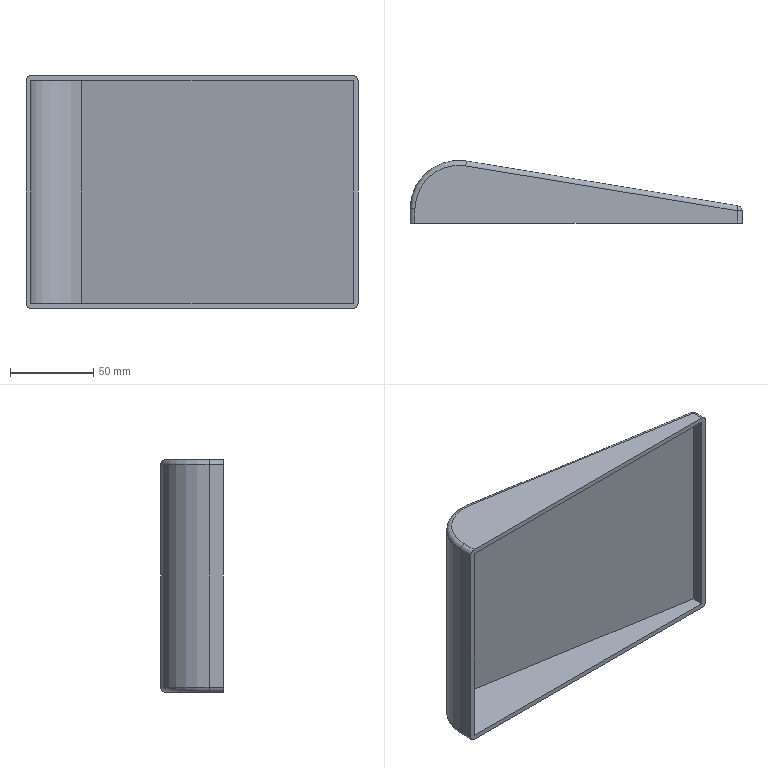Part | SolidWorks | features BaseBody 1 | 1 solid | 24 faces | box 200 x 37.759 x 140 mm | volume 122488 mm3 | plane 11 | cylinder 9 | torus 2 | sphere 2 | commonest cylinder face diameters 6 x7 52.553 x1 58.553 x1
STEP:
#1=CARTESIAN_POINT('',(200.,0.,137.));
#2=VERTEX_POINT('',#1);
#3=CARTESIAN_POINT('',(200.,0.,3.));
#4=VERTEX_POINT('',#3);
#5=CARTESIAN_POINT('',(200.,0.,140.));
#6=DIRECTION('',(0.,0.,-1.));
#7=VECTOR('',#6,1000.);
#8=LINE('',#5,#7);
#9=EDGE_CURVE('',#2,#4,#8,.T.);
#10=ORIENTED_EDGE('',*,*,#9,.F.);
#11=CARTESIAN_POINT('',(197.,0.,140.));
#12=VERTEX_POINT('',#11);
#13=CARTESIAN_POINT('',(197.,0.,137.));
#14=DIRECTION('',(0.,-1.,0.));
#15=DIRECTION('',(-1.,0.,0.));
#16=AXIS2_PLACEMENT_3D('',#13,#14,#15);
#17=CIRCLE('',#16,3.);
#18=EDGE_CURVE('',#2,#12,#17,.T.);
#19=ORIENTED_EDGE('',*,*,#18,.T.);
#20=CARTESIAN_POINT('',(3.,0.,140.));
#21=VERTEX_POINT('',#20);
#22=CARTESIAN_POINT('',(200.,0.,140.));
#23=DIRECTION('',(1.,0.,0.));
#24=VECTOR('',#23,1000.);
#25=LINE('',#22,#24);
#26=EDGE_CURVE('',#21,#12,#25,.T.);
#27=ORIENTED_EDGE('',*,*,#26,.F.);
#28=CARTESIAN_POINT('',(0.,0.,137.));
#29=VERTEX_POINT('',#28);
#30=CARTESIAN_POINT('',(3.,0.,137.));
#31=DIRECTION('',(0.,-1.,0.));
#32=DIRECTION('',(-1.,0.,0.));
#33=AXIS2_PLACEMENT_3D('',#30,#31,#32);
#34=CIRCLE('',#33,3.);
#35=EDGE_CURVE('',#21,#29,#34,.T.);
#36=ORIENTED_EDGE('',*,*,#35,.T.);
#37=CARTESIAN_POINT('',(0.,0.,3.));
#38=VERTEX_POINT('',#37);
#39=CARTESIAN_POINT('',(0.,0.,140.));
#40=DIRECTION('',(0.,0.,-1.));
#41=VECTOR('',#40,1000.);
#42=LINE('',#39,#41);
#43=EDGE_CURVE('',#29,#38,#42,.T.);
#44=ORIENTED_EDGE('',*,*,#43,.T.);
#45=CARTESIAN_POINT('',(3.,0.,0.));
#46=VERTEX_POINT('',#45);
#47=CARTESIAN_POINT('',(3.,0.,3.));
#48=DIRECTION('',(0.,-1.,0.));
#49=DIRECTION('',(-1.,0.,0.));
#50=AXIS2_PLACEMENT_3D('',#47,#48,#49);
#51=CIRCLE('',#50,3.);
#52=EDGE_CURVE('',#38,#46,#51,.T.);
#53=ORIENTED_EDGE('',*,*,#52,.T.);
#54=CARTESIAN_POINT('',(197.,0.,0.));
#55=VERTEX_POINT('',#54);
#56=CARTESIAN_POINT('',(200.,0.,0.));
#57=DIRECTION('',(1.,0.,0.));
#58=VECTOR('',#57,1000.);
#59=LINE('',#56,#58);
#60=EDGE_CURVE('',#46,#55,#59,.T.);
#61=ORIENTED_EDGE('',*,*,#60,.T.);
#62=CARTESIAN_POINT('',(197.,0.,3.));
#63=DIRECTION('',(0.,-1.,0.));
#64=DIRECTION('',(-1.,0.,0.));
#65=AXIS2_PLACEMENT_3D('',#62,#63,#64);
#66=CIRCLE('',#65,3.);
#67=EDGE_CURVE('',#55,#4,#66,.T.);
#68=ORIENTED_EDGE('',*,*,#67,.T.);
#69=EDGE_LOOP('',(#10,#19,#27,#36,#44,#53,#61,#68));
#70=FACE_OUTER_BOUND('',#69,.T.);
#71=CARTESIAN_POINT('',(3.,0.,3.));
#72=VERTEX_POINT('',#71);
#73=CARTESIAN_POINT('',(197.,0.,3.));
#74=VERTEX_POINT('',#73);
#75=CARTESIAN_POINT('',(29.276,0.,3.));
#76=DIRECTION('',(1.,0.,0.));
#77=VECTOR('',#76,1000.);
#78=LINE('',#75,#77);
#79=EDGE_CURVE('',#72,#74,#78,.T.);
#80=ORIENTED_EDGE('',*,*,#79,.F.);
#81=CARTESIAN_POINT('',(3.,0.,137.));
#82=VERTEX_POINT('',#81);
#83=CARTESIAN_POINT('',(3.,0.,140.));
#84=DIRECTION('',(0.,0.,-1.));
#85=VECTOR('',#84,1000.);
#86=LINE('',#83,#85);
#87=EDGE_CURVE('',#82,#72,#86,.T.);
#88=ORIENTED_EDGE('',*,*,#87,.F.);
#89=CARTESIAN_POINT('',(197.,0.,137.));
#90=VERTEX_POINT('',#89);
#91=CARTESIAN_POINT('',(29.276,0.,137.));
#92=DIRECTION('',(1.,0.,0.));
#93=VECTOR('',#92,1000.);
#94=LINE('',#91,#93);
#95=EDGE_CURVE('',#82,#90,#94,.T.);
#96=ORIENTED_EDGE('',*,*,#95,.T.);
#97=CARTESIAN_POINT('',(197.,0.,140.));
#98=DIRECTION('',(0.,0.,-1.));
#99=VECTOR('',#98,1000.);
#100=LINE('',#97,#99);
#101=EDGE_CURVE('',#90,#74,#100,.T.);
#102=ORIENTED_EDGE('',*,*,#101,.T.);
#103=EDGE_LOOP('',(#80,#88,#96,#102));
#104=FACE_BOUND('',#103,.T.);
#105=CARTESIAN_POINT('',(200.,0.,140.));
#106=DIRECTION('',(0.,1.,0.));
#107=DIRECTION('',(-1.,0.,0.));
#108=AXIS2_PLACEMENT_3D('',#105,#106,#107);
#109=PLANE('',#108);
#110=ADVANCED_FACE('',(#70,#104),#109,.F.);
#111=CARTESIAN_POINT('',(200.,7.454,3.));
#112=VERTEX_POINT('',#111);
#113=CARTESIAN_POINT('',(200.,7.454,137.));
#114=VERTEX_POINT('',#113);
#115=CARTESIAN_POINT('',(200.,7.454,140.));
#116=DIRECTION('',(0.,0.,1.));
#117=VECTOR('',#116,1000.);
#118=LINE('',#115,#117);
#119=EDGE_CURVE('',#112,#114,#118,.T.);
#120=ORIENTED_EDGE('',*,*,#119,.T.);
#121=CARTESIAN_POINT('',(200.,10.,137.));
#122=DIRECTION('',(0.,-1.,0.));
#123=VECTOR('',#122,1000.);
#124=LINE('',#121,#123);
#125=EDGE_CURVE('',#114,#2,#124,.T.);
#126=ORIENTED_EDGE('',*,*,#125,.T.);
#127=ORIENTED_EDGE('',*,*,#9,.T.);
#128=CARTESIAN_POINT('',(200.,7.454,3.));
#129=DIRECTION('',(0.,1.,0.));
#130=VECTOR('',#129,1000.);
#131=LINE('',#128,#130);
#132=EDGE_CURVE('',#4,#112,#131,.T.);
#133=ORIENTED_EDGE('',*,*,#132,.T.);
#134=EDGE_LOOP('',(#120,#126,#127,#133));
#135=FACE_OUTER_BOUND('',#134,.T.);
#136=CARTESIAN_POINT('',(200.,10.,140.));
#137=DIRECTION('',(-1.,0.,0.));
#138=DIRECTION('',(0.,0.,1.));
#139=AXIS2_PLACEMENT_3D('',#136,#137,#138);
#140=PLANE('',#139);
#141=ADVANCED_FACE('',(#135),#140,.F.);
#142=CARTESIAN_POINT('',(34.04,37.369,137.));
#143=VERTEX_POINT('',#142);
#144=CARTESIAN_POINT('',(34.04,37.369,3.));
#145=VERTEX_POINT('',#144);
#146=CARTESIAN_POINT('',(34.04,37.369,140.));
#147=DIRECTION('',(0.,0.,-1.));
#148=VECTOR('',#147,1000.);
#149=LINE('',#146,#148);
#150=EDGE_CURVE('',#143,#145,#149,.T.);
#151=ORIENTED_EDGE('',*,*,#150,.F.);
#152=CARTESIAN_POINT('',(197.488,10.414,137.));
#153=VERTEX_POINT('',#152);
#154=CARTESIAN_POINT('',(34.04,37.369,137.));
#155=DIRECTION('',(0.9867,-0.1627,0.));
#156=VECTOR('',#155,1000.);
#157=LINE('',#154,#156);
#158=EDGE_CURVE('',#143,#153,#157,.T.);
#159=ORIENTED_EDGE('',*,*,#158,.T.);
#160=CARTESIAN_POINT('',(197.488,10.414,3.));
#161=VERTEX_POINT('',#160);
#162=CARTESIAN_POINT('',(197.488,10.414,140.));
#163=DIRECTION('',(0.,0.,-1.));
#164=VECTOR('',#163,1000.);
#165=LINE('',#162,#164);
#166=EDGE_CURVE('',#153,#161,#165,.T.);
#167=ORIENTED_EDGE('',*,*,#166,.T.);
#168=CARTESIAN_POINT('',(34.04,37.369,3.));
#169=DIRECTION('',(-0.9867,0.1627,0.));
#170=VECTOR('',#169,1000.);
#171=LINE('',#168,#170);
#172=EDGE_CURVE('',#161,#145,#171,.T.);
#173=ORIENTED_EDGE('',*,*,#172,.T.);
#174=EDGE_LOOP('',(#151,#159,#167,#173));
#175=FACE_OUTER_BOUND('',#174,.T.);
#176=CARTESIAN_POINT('',(34.04,37.369,140.));
#177=DIRECTION('',(-0.1627,-0.9867,0.));
#178=DIRECTION('',(0.9867,-0.1627,0.));
#179=AXIS2_PLACEMENT_3D('',#176,#177,#178);
#180=PLANE('',#179);
#181=ADVANCED_FACE('',(#175),#180,.F.);
#182=CARTESIAN_POINT('',(0.,8.482,137.));
#183=VERTEX_POINT('',#182);
#184=CARTESIAN_POINT('',(0.,8.482,3.));
#185=VERTEX_POINT('',#184);
#186=CARTESIAN_POINT('',(0.,8.482,140.));
#187=DIRECTION('',(0.,0.,-1.));
#188=VECTOR('',#187,1000.);
#189=LINE('',#186,#188);
#190=EDGE_CURVE('',#183,#185,#189,.T.);
#191=ORIENTED_EDGE('',*,*,#190,.F.);
#192=CARTESIAN_POINT('',(29.276,8.482,137.));
#193=DIRECTION('',(0.,0.,-1.));
#194=DIRECTION('',(-1.,0.,0.));
#195=AXIS2_PLACEMENT_3D('',#192,#193,#194);
#196=CIRCLE('',#195,29.276);
#197=EDGE_CURVE('',#183,#143,#196,.T.);
#198=ORIENTED_EDGE('',*,*,#197,.T.);
#199=ORIENTED_EDGE('',*,*,#150,.T.);
#200=CARTESIAN_POINT('',(29.276,8.482,3.));
#201=DIRECTION('',(0.,0.,1.));
#202=DIRECTION('',(-1.,0.,0.));
#203=AXIS2_PLACEMENT_3D('',#200,#201,#202);
#204=CIRCLE('',#203,29.276);
#205=EDGE_CURVE('',#145,#185,#204,.T.);
#206=ORIENTED_EDGE('',*,*,#205,.T.);
#207=EDGE_LOOP('',(#191,#198,#199,#206));
#208=FACE_OUTER_BOUND('',#207,.T.);
#209=CARTESIAN_POINT('',(29.276,8.482,140.));
#210=DIRECTION('',(0.,0.,-1.));
#211=DIRECTION('',(-1.,0.,0.));
#212=AXIS2_PLACEMENT_3D('',#209,#210,#211);
#213=CYLINDRICAL_SURFACE('',#212,29.276);
#214=ADVANCED_FACE('',(#208),#213,.T.);
#215=ORIENTED_EDGE('',*,*,#43,.F.);
#216=CARTESIAN_POINT('',(0.,0.,137.));
#217=DIRECTION('',(0.,1.,0.));
#218=VECTOR('',#217,1000.);
#219=LINE('',#216,#218);
#220=EDGE_CURVE('',#29,#183,#219,.T.);
#221=ORIENTED_EDGE('',*,*,#220,.T.);
#222=ORIENTED_EDGE('',*,*,#190,.T.);
#223=CARTESIAN_POINT('',(0.,0.,3.));
#224=DIRECTION('',(0.,-1.,0.));
#225=VECTOR('',#224,1000.);
#226=LINE('',#223,#225);
#227=EDGE_CURVE('',#185,#38,#226,.T.);
#228=ORIENTED_EDGE('',*,*,#227,.T.);
#229=EDGE_LOOP('',(#215,#221,#222,#228));
#230=FACE_OUTER_BOUND('',#229,.T.);
#231=CARTESIAN_POINT('',(0.,0.,140.));
#232=DIRECTION('',(1.,0.,0.));
#233=DIRECTION('',(0.,0.,-1.));
#234=AXIS2_PLACEMENT_3D('',#231,#232,#233);
#235=PLANE('',#234);
#236=ADVANCED_FACE('',(#230),#235,.F.);
#237=ORIENTED_EDGE('',*,*,#26,.T.);
#238=CARTESIAN_POINT('',(197.,7.454,140.));
#239=VERTEX_POINT('',#238);
#240=CARTESIAN_POINT('',(197.,8.482,140.));
#241=DIRECTION('',(0.,1.,0.));
#242=VECTOR('',#241,1000.);
#243=LINE('',#240,#242);
#244=EDGE_CURVE('',#12,#239,#243,.T.);
#245=ORIENTED_EDGE('',*,*,#244,.T.);
#246=CARTESIAN_POINT('',(33.552,34.409,140.));
#247=VERTEX_POINT('',#246);
#248=CARTESIAN_POINT('',(33.552,34.409,140.));
#249=DIRECTION('',(-0.9867,0.1627,0.));
#250=VECTOR('',#249,1000.);
#251=LINE('',#248,#250);
#252=EDGE_CURVE('',#239,#247,#251,.T.);
#253=ORIENTED_EDGE('',*,*,#252,.T.);
#254=CARTESIAN_POINT('',(3.,8.482,140.));
#255=VERTEX_POINT('',#254);
#256=CARTESIAN_POINT('',(29.276,8.482,140.));
#257=DIRECTION('',(0.,0.,1.));
#258=DIRECTION('',(-1.,0.,0.));
#259=AXIS2_PLACEMENT_3D('',#256,#257,#258);
#260=CIRCLE('',#259,26.276);
#261=EDGE_CURVE('',#247,#255,#260,.T.);
#262=ORIENTED_EDGE('',*,*,#261,.T.);
#263=CARTESIAN_POINT('',(3.,8.482,140.));
#264=DIRECTION('',(0.,-1.,0.));
#265=VECTOR('',#264,1000.);
#266=LINE('',#263,#265);
#267=EDGE_CURVE('',#255,#21,#266,.T.);
#268=ORIENTED_EDGE('',*,*,#267,.T.);
#269=EDGE_LOOP('',(#237,#245,#253,#262,#268));
#270=FACE_OUTER_BOUND('',#269,.T.);
#271=CARTESIAN_POINT('',(29.276,8.482,140.));
#272=DIRECTION('',(0.,0.,-1.));
#273=DIRECTION('',(-1.,0.,0.));
#274=AXIS2_PLACEMENT_3D('',#271,#272,#273);
#275=PLANE('',#274);
#276=ADVANCED_FACE('',(#270),#275,.F.);
#277=CARTESIAN_POINT('',(33.552,34.409,0.));
#278=VERTEX_POINT('',#277);
#279=CARTESIAN_POINT('',(197.,7.454,0.));
#280=VERTEX_POINT('',#279);
#281=CARTESIAN_POINT('',(197.,7.454,0.));
#282=DIRECTION('',(0.9867,-0.1627,0.));
#283=VECTOR('',#282,1000.);
#284=LINE('',#281,#283);
#285=EDGE_CURVE('',#278,#280,#284,.T.);
#286=ORIENTED_EDGE('',*,*,#285,.T.);
#287=CARTESIAN_POINT('',(197.,0.,0.));
#288=DIRECTION('',(0.,-1.,0.));
#289=VECTOR('',#288,1000.);
#290=LINE('',#287,#289);
#291=EDGE_CURVE('',#280,#55,#290,.T.);
#292=ORIENTED_EDGE('',*,*,#291,.T.);
#293=ORIENTED_EDGE('',*,*,#60,.F.);
#294=CARTESIAN_POINT('',(3.,8.482,0.));
#295=VERTEX_POINT('',#294);
#296=CARTESIAN_POINT('',(3.,8.482,0.));
#297=DIRECTION('',(0.,1.,0.));
#298=VECTOR('',#297,1000.);
#299=LINE('',#296,#298);
#300=EDGE_CURVE('',#46,#295,#299,.T.);
#301=ORIENTED_EDGE('',*,*,#300,.T.);
#302=CARTESIAN_POINT('',(29.276,8.482,0.));
#303=DIRECTION('',(0.,0.,-1.));
#304=DIRECTION('',(-1.,0.,0.));
#305=AXIS2_PLACEMENT_3D('',#302,#303,#304);
#306=CIRCLE('',#305,26.276);
#307=EDGE_CURVE('',#295,#278,#306,.T.);
#308=ORIENTED_EDGE('',*,*,#307,.T.);
#309=EDGE_LOOP('',(#286,#292,#293,#301,#308));
#310=FACE_OUTER_BOUND('',#309,.T.);
#311=CARTESIAN_POINT('',(29.276,8.482,0.));
#312=DIRECTION('',(0.,0.,-1.));
#313=DIRECTION('',(-1.,0.,0.));
#314=AXIS2_PLACEMENT_3D('',#311,#312,#313);
#315=PLANE('',#314);
#316=ADVANCED_FACE('',(#310),#315,.T.);
#317=CARTESIAN_POINT('',(197.,7.454,3.));
#318=VERTEX_POINT('',#317);
#319=CARTESIAN_POINT('',(197.,8.482,3.));
#320=DIRECTION('',(0.,1.,0.));
#321=VECTOR('',#320,1000.);
#322=LINE('',#319,#321);
#323=EDGE_CURVE('',#74,#318,#322,.T.);
#324=ORIENTED_EDGE('',*,*,#323,.F.);
#325=ORIENTED_EDGE('',*,*,#101,.F.);
#326=CARTESIAN_POINT('',(197.,7.454,137.));
#327=VERTEX_POINT('',#326);
#328=CARTESIAN_POINT('',(197.,8.482,137.));
#329=DIRECTION('',(0.,1.,0.));
#330=VECTOR('',#329,1000.);
#331=LINE('',#328,#330);
#332=EDGE_CURVE('',#90,#327,#331,.T.);
#333=ORIENTED_EDGE('',*,*,#332,.T.);
#334=CARTESIAN_POINT('',(197.,7.454,140.));
#335=DIRECTION('',(0.,0.,-1.));
#336=VECTOR('',#335,1000.);
#337=LINE('',#334,#336);
#338=EDGE_CURVE('',#327,#318,#337,.T.);
#339=ORIENTED_EDGE('',*,*,#338,.T.);
#340=EDGE_LOOP('',(#324,#325,#333,#339));
#341=FACE_OUTER_BOUND('',#340,.T.);
#342=CARTESIAN_POINT('',(197.,10.,140.));
#343=DIRECTION('',(-1.,0.,0.));
#344=DIRECTION('',(0.,0.,1.));
#345=AXIS2_PLACEMENT_3D('',#342,#343,#344);
#346=PLANE('',#345);
#347=ADVANCED_FACE('',(#341),#346,.T.);
#348=CARTESIAN_POINT('',(33.552,34.409,3.));
#349=VERTEX_POINT('',#348);
#350=CARTESIAN_POINT('',(33.552,34.409,3.));
#351=DIRECTION('',(-0.9867,0.1627,0.));
#352=VECTOR('',#351,1000.);
#353=LINE('',#350,#352);
#354=EDGE_CURVE('',#318,#349,#353,.T.);
#355=ORIENTED_EDGE('',*,*,#354,.F.);
#356=ORIENTED_EDGE('',*,*,#338,.F.);
#357=CARTESIAN_POINT('',(33.552,34.409,137.));
#358=VERTEX_POINT('',#357);
#359=CARTESIAN_POINT('',(33.552,34.409,137.));
#360=DIRECTION('',(-0.9867,0.1627,0.));
#361=VECTOR('',#360,1000.);
#362=LINE('',#359,#361);
#363=EDGE_CURVE('',#327,#358,#362,.T.);
#364=ORIENTED_EDGE('',*,*,#363,.T.);
#365=CARTESIAN_POINT('',(33.552,34.409,140.));
#366=DIRECTION('',(0.,0.,-1.));
#367=VECTOR('',#366,1000.);
#368=LINE('',#365,#367);
#369=EDGE_CURVE('',#358,#349,#368,.T.);
#370=ORIENTED_EDGE('',*,*,#369,.T.);
#371=EDGE_LOOP('',(#355,#356,#364,#370));
#372=FACE_OUTER_BOUND('',#371,.T.);
#373=CARTESIAN_POINT('',(33.552,34.409,140.));
#374=DIRECTION('',(-0.1627,-0.9867,0.));
#375=DIRECTION('',(0.9867,-0.1627,0.));
#376=AXIS2_PLACEMENT_3D('',#373,#374,#375);
#377=PLANE('',#376);
#378=ADVANCED_FACE('',(#372),#377,.T.);
#379=CARTESIAN_POINT('',(3.,8.482,3.));
#380=VERTEX_POINT('',#379);
#381=CARTESIAN_POINT('',(29.276,8.482,3.));
#382=DIRECTION('',(0.,0.,1.));
#383=DIRECTION('',(-1.,0.,0.));
#384=AXIS2_PLACEMENT_3D('',#381,#382,#383);
#385=CIRCLE('',#384,26.276);
#386=EDGE_CURVE('',#349,#380,#385,.T.);
#387=ORIENTED_EDGE('',*,*,#386,.F.);
#388=ORIENTED_EDGE('',*,*,#369,.F.);
#389=CARTESIAN_POINT('',(3.,8.482,137.));
#390=VERTEX_POINT('',#389);
#391=CARTESIAN_POINT('',(29.276,8.482,137.));
#392=DIRECTION('',(0.,0.,1.));
#393=DIRECTION('',(-1.,0.,0.));
#394=AXIS2_PLACEMENT_3D('',#391,#392,#393);
#395=CIRCLE('',#394,26.276);
#396=EDGE_CURVE('',#358,#390,#395,.T.);
#397=ORIENTED_EDGE('',*,*,#396,.T.);
#398=CARTESIAN_POINT('',(3.,8.482,140.));
#399=DIRECTION('',(0.,0.,-1.));
#400=VECTOR('',#399,1000.);
#401=LINE('',#398,#400);
#402=EDGE_CURVE('',#390,#380,#401,.T.);
#403=ORIENTED_EDGE('',*,*,#402,.T.);
#404=EDGE_LOOP('',(#387,#388,#397,#403));
#405=FACE_OUTER_BOUND('',#404,.T.);
#406=CARTESIAN_POINT('',(29.276,8.482,140.));
#407=DIRECTION('',(0.,0.,-1.));
#408=DIRECTION('',(-1.,0.,0.));
#409=AXIS2_PLACEMENT_3D('',#406,#407,#408);
#410=CYLINDRICAL_SURFACE('',#409,26.276);
#411=ADVANCED_FACE('',(#405),#410,.F.);
#412=CARTESIAN_POINT('',(3.,8.482,3.));
#413=DIRECTION('',(0.,-1.,0.));
#414=VECTOR('',#413,1000.);
#415=LINE('',#412,#414);
#416=EDGE_CURVE('',#380,#72,#415,.T.);
#417=ORIENTED_EDGE('',*,*,#416,.F.);
#418=ORIENTED_EDGE('',*,*,#402,.F.);
#419=CARTESIAN_POINT('',(3.,8.482,137.));
#420=DIRECTION('',(0.,-1.,0.));
#421=VECTOR('',#420,1000.);
#422=LINE('',#419,#421);
#423=EDGE_CURVE('',#390,#82,#422,.T.);
#424=ORIENTED_EDGE('',*,*,#423,.T.);
#425=ORIENTED_EDGE('',*,*,#87,.T.);
#426=EDGE_LOOP('',(#417,#418,#424,#425));
#427=FACE_OUTER_BOUND('',#426,.T.);
#428=CARTESIAN_POINT('',(3.,0.,140.));
#429=DIRECTION('',(1.,0.,0.));
#430=DIRECTION('',(0.,0.,-1.));
#431=AXIS2_PLACEMENT_3D('',#428,#429,#430);
#432=PLANE('',#431);
#433=ADVANCED_FACE('',(#427),#432,.T.);
#434=ORIENTED_EDGE('',*,*,#95,.F.);
#435=ORIENTED_EDGE('',*,*,#423,.F.);
#436=ORIENTED_EDGE('',*,*,#396,.F.);
#437=ORIENTED_EDGE('',*,*,#363,.F.);
#438=ORIENTED_EDGE('',*,*,#332,.F.);
#439=EDGE_LOOP('',(#434,#435,#436,#437,#438));
#440=FACE_OUTER_BOUND('',#439,.T.);
#441=CARTESIAN_POINT('',(29.276,8.482,137.));
#442=DIRECTION('',(0.,0.,-1.));
#443=DIRECTION('',(-1.,0.,0.));
#444=AXIS2_PLACEMENT_3D('',#441,#442,#443);
#445=PLANE('',#444);
#446=ADVANCED_FACE('',(#440),#445,.T.);
#447=ORIENTED_EDGE('',*,*,#79,.T.);
#448=ORIENTED_EDGE('',*,*,#323,.T.);
#449=ORIENTED_EDGE('',*,*,#354,.T.);
#450=ORIENTED_EDGE('',*,*,#386,.T.);
#451=ORIENTED_EDGE('',*,*,#416,.T.);
#452=EDGE_LOOP('',(#447,#448,#449,#450,#451));
#453=FACE_OUTER_BOUND('',#452,.T.);
#454=CARTESIAN_POINT('',(29.276,8.482,3.));
#455=DIRECTION('',(0.,0.,-1.));
#456=DIRECTION('',(-1.,0.,0.));
#457=AXIS2_PLACEMENT_3D('',#454,#455,#456);
#458=PLANE('',#457);
#459=ADVANCED_FACE('',(#453),#458,.F.);
#460=ORIENTED_EDGE('',*,*,#166,.F.);
#461=CARTESIAN_POINT('',(197.,7.454,137.));
#462=DIRECTION('',(0.,0.,-1.));
#463=DIRECTION('',(-1.,0.,0.));
#464=AXIS2_PLACEMENT_3D('',#461,#462,#463);
#465=CIRCLE('',#464,3.);
#466=EDGE_CURVE('',#153,#114,#465,.T.);
#467=ORIENTED_EDGE('',*,*,#466,.T.);
#468=ORIENTED_EDGE('',*,*,#119,.F.);
#469=CARTESIAN_POINT('',(197.,7.454,3.));
#470=DIRECTION('',(0.,0.,1.));
#471=DIRECTION('',(-1.,0.,0.));
#472=AXIS2_PLACEMENT_3D('',#469,#470,#471);
#473=CIRCLE('',#472,3.);
#474=EDGE_CURVE('',#112,#161,#473,.T.);
#475=ORIENTED_EDGE('',*,*,#474,.T.);
#476=EDGE_LOOP('',(#460,#467,#468,#475));
#477=FACE_OUTER_BOUND('',#476,.T.);
#478=CARTESIAN_POINT('',(197.,7.454,140.));
#479=DIRECTION('',(0.,0.,-1.));
#480=DIRECTION('',(-1.,0.,0.));
#481=AXIS2_PLACEMENT_3D('',#478,#479,#480);
#482=CYLINDRICAL_SURFACE('',#481,3.);
#483=ADVANCED_FACE('',(#477),#482,.T.);
#484=ORIENTED_EDGE('',*,*,#35,.F.);
#485=ORIENTED_EDGE('',*,*,#267,.F.);
#486=CARTESIAN_POINT('',(3.,8.482,137.));
#487=DIRECTION('',(0.,1.,0.));
#488=DIRECTION('',(0.,0.,1.));
#489=AXIS2_PLACEMENT_3D('',#486,#487,#488);
#490=CIRCLE('',#489,3.);
#491=EDGE_CURVE('',#183,#255,#490,.T.);
#492=ORIENTED_EDGE('',*,*,#491,.F.);
#493=ORIENTED_EDGE('',*,*,#220,.F.);
#494=EDGE_LOOP('',(#484,#485,#492,#493));
#495=FACE_OUTER_BOUND('',#494,.T.);
#496=CARTESIAN_POINT('',(3.,8.482,137.));
#497=DIRECTION('',(0.,-1.,0.));
#498=DIRECTION('',(0.,0.,-1.));
#499=AXIS2_PLACEMENT_3D('',#496,#497,#498);
#500=CYLINDRICAL_SURFACE('',#499,3.);
#501=ADVANCED_FACE('',(#495),#500,.T.);
#502=ORIENTED_EDGE('',*,*,#491,.T.);
#503=ORIENTED_EDGE('',*,*,#261,.F.);
#504=CARTESIAN_POINT('',(33.552,34.409,137.));
#505=DIRECTION('',(0.9867,-0.1627,0.));
#506=DIRECTION('',(0.1627,0.9867,0.));
#507=AXIS2_PLACEMENT_3D('',#504,#505,#506);
#508=CIRCLE('',#507,3.);
#509=EDGE_CURVE('',#143,#247,#508,.T.);
#510=ORIENTED_EDGE('',*,*,#509,.F.);
#511=ORIENTED_EDGE('',*,*,#197,.F.);
#512=EDGE_LOOP('',(#502,#503,#510,#511));
#513=FACE_OUTER_BOUND('',#512,.T.);
#514=CARTESIAN_POINT('',(29.276,8.482,137.));
#515=DIRECTION('',(0.,0.,-1.));
#516=DIRECTION('',(-1.,0.,0.));
#517=AXIS2_PLACEMENT_3D('',#514,#515,#516);
#518=TOROIDAL_SURFACE('',#517,26.276,3.);
#519=ADVANCED_FACE('',(#513),#518,.T.);
#520=CARTESIAN_POINT('',(197.,7.454,137.));
#521=DIRECTION('',(0.9867,-0.1627,0.));
#522=DIRECTION('',(0.1627,0.9867,0.));
#523=AXIS2_PLACEMENT_3D('',#520,#521,#522);
#524=CIRCLE('',#523,3.);
#525=EDGE_CURVE('',#153,#239,#524,.T.);
#526=ORIENTED_EDGE('',*,*,#525,.F.);
#527=ORIENTED_EDGE('',*,*,#158,.F.);
#528=ORIENTED_EDGE('',*,*,#509,.T.);
#529=ORIENTED_EDGE('',*,*,#252,.F.);
#530=EDGE_LOOP('',(#526,#527,#528,#529));
#531=FACE_OUTER_BOUND('',#530,.T.);
#532=CARTESIAN_POINT('',(33.552,34.409,137.));
#533=DIRECTION('',(-0.9867,0.1627,0.));
#534=DIRECTION('',(-0.1627,-0.9867,0.));
#535=AXIS2_PLACEMENT_3D('',#532,#533,#534);
#536=CYLINDRICAL_SURFACE('',#535,3.);
#537=ADVANCED_FACE('',(#531),#536,.T.);
#538=ORIENTED_EDGE('',*,*,#466,.F.);
#539=ORIENTED_EDGE('',*,*,#525,.T.);
#540=CARTESIAN_POINT('',(197.,7.454,137.));
#541=DIRECTION('',(0.,-1.,0.));
#542=DIRECTION('',(0.,0.,-1.));
#543=AXIS2_PLACEMENT_3D('',#540,#541,#542);
#544=CIRCLE('',#543,3.);
#545=EDGE_CURVE('',#114,#239,#544,.T.);
#546=ORIENTED_EDGE('',*,*,#545,.F.);
#547=EDGE_LOOP('',(#538,#539,#546));
#548=FACE_OUTER_BOUND('',#547,.T.);
#549=CARTESIAN_POINT('',(197.,7.454,137.));
#550=DIRECTION('',(0.,1.,0.));
#551=DIRECTION('',(-1.,0.,0.));
#552=AXIS2_PLACEMENT_3D('',#549,#550,#551);
#553=SPHERICAL_SURFACE('',#552,3.);
#554=ADVANCED_FACE('',(#548),#553,.T.);
#555=ORIENTED_EDGE('',*,*,#18,.F.);
#556=ORIENTED_EDGE('',*,*,#125,.F.);
#557=ORIENTED_EDGE('',*,*,#545,.T.);
#558=ORIENTED_EDGE('',*,*,#244,.F.);
#559=EDGE_LOOP('',(#555,#556,#557,#558));
#560=FACE_OUTER_BOUND('',#559,.T.);
#561=CARTESIAN_POINT('',(197.,8.482,137.));
#562=DIRECTION('',(0.,1.,0.));
#563=DIRECTION('',(0.,0.,1.));
#564=AXIS2_PLACEMENT_3D('',#561,#562,#563);
#565=CYLINDRICAL_SURFACE('',#564,3.);
#566=ADVANCED_FACE('',(#560),#565,.T.);
#567=ORIENTED_EDGE('',*,*,#52,.F.);
#568=ORIENTED_EDGE('',*,*,#227,.F.);
#569=CARTESIAN_POINT('',(3.,8.482,3.));
#570=DIRECTION('',(0.,1.,0.));
#571=DIRECTION('',(0.,0.,1.));
#572=AXIS2_PLACEMENT_3D('',#569,#570,#571);
#573=CIRCLE('',#572,3.);
#574=EDGE_CURVE('',#295,#185,#573,.T.);
#575=ORIENTED_EDGE('',*,*,#574,.F.);
#576=ORIENTED_EDGE('',*,*,#300,.F.);
#577=EDGE_LOOP('',(#567,#568,#575,#576));
#578=FACE_OUTER_BOUND('',#577,.T.);
#579=CARTESIAN_POINT('',(3.,0.,3.));
#580=DIRECTION('',(0.,1.,0.));
#581=DIRECTION('',(0.,0.,1.));
#582=AXIS2_PLACEMENT_3D('',#579,#580,#581);
#583=CYLINDRICAL_SURFACE('',#582,3.);
#584=ADVANCED_FACE('',(#578),#583,.T.);
#585=ORIENTED_EDGE('',*,*,#574,.T.);
#586=ORIENTED_EDGE('',*,*,#205,.F.);
#587=CARTESIAN_POINT('',(33.552,34.409,3.));
#588=DIRECTION('',(0.9867,-0.1627,0.));
#589=DIRECTION('',(0.1627,0.9867,0.));
#590=AXIS2_PLACEMENT_3D('',#587,#588,#589);
#591=CIRCLE('',#590,3.);
#592=EDGE_CURVE('',#278,#145,#591,.T.);
#593=ORIENTED_EDGE('',*,*,#592,.F.);
#594=ORIENTED_EDGE('',*,*,#307,.F.);
#595=EDGE_LOOP('',(#585,#586,#593,#594));
#596=FACE_OUTER_BOUND('',#595,.T.);
#597=CARTESIAN_POINT('',(29.276,8.482,3.));
#598=DIRECTION('',(0.,0.,-1.));
#599=DIRECTION('',(-1.,0.,0.));
#600=AXIS2_PLACEMENT_3D('',#597,#598,#599);
#601=TOROIDAL_SURFACE('',#600,26.276,3.);
#602=ADVANCED_FACE('',(#596),#601,.T.);
#603=ORIENTED_EDGE('',*,*,#592,.T.);
#604=ORIENTED_EDGE('',*,*,#172,.F.);
#605=CARTESIAN_POINT('',(197.,7.454,3.));
#606=DIRECTION('',(0.9867,-0.1627,0.));
#607=DIRECTION('',(0.1627,0.9867,0.));
#608=AXIS2_PLACEMENT_3D('',#605,#606,#607);
#609=CIRCLE('',#608,3.);
#610=EDGE_CURVE('',#280,#161,#609,.T.);
#611=ORIENTED_EDGE('',*,*,#610,.F.);
#612=ORIENTED_EDGE('',*,*,#285,.F.);
#613=EDGE_LOOP('',(#603,#604,#611,#612));
#614=FACE_OUTER_BOUND('',#613,.T.);
#615=CARTESIAN_POINT('',(33.552,34.409,3.));
#616=DIRECTION('',(0.9867,-0.1627,0.));
#617=DIRECTION('',(0.1627,0.9867,0.));
#618=AXIS2_PLACEMENT_3D('',#615,#616,#617);
#619=CYLINDRICAL_SURFACE('',#618,3.);
#620=ADVANCED_FACE('',(#614),#619,.T.);
#621=ORIENTED_EDGE('',*,*,#610,.T.);
#622=ORIENTED_EDGE('',*,*,#474,.F.);
#623=CARTESIAN_POINT('',(197.,7.454,3.));
#624=DIRECTION('',(0.,-1.,0.));
#625=DIRECTION('',(0.,0.,-1.));
#626=AXIS2_PLACEMENT_3D('',#623,#624,#625);
#627=CIRCLE('',#626,3.);
#628=EDGE_CURVE('',#280,#112,#627,.T.);
#629=ORIENTED_EDGE('',*,*,#628,.F.);
#630=EDGE_LOOP('',(#621,#622,#629));
#631=FACE_OUTER_BOUND('',#630,.T.);
#632=CARTESIAN_POINT('',(197.,7.454,3.));
#633=DIRECTION('',(0.,1.,0.));
#634=DIRECTION('',(-1.,0.,0.));
#635=AXIS2_PLACEMENT_3D('',#632,#633,#634);
#636=SPHERICAL_SURFACE('',#635,3.);
#637=ADVANCED_FACE('',(#631),#636,.T.);
#638=ORIENTED_EDGE('',*,*,#67,.F.);
#639=ORIENTED_EDGE('',*,*,#291,.F.);
#640=ORIENTED_EDGE('',*,*,#628,.T.);
#641=ORIENTED_EDGE('',*,*,#132,.F.);
#642=EDGE_LOOP('',(#638,#639,#640,#641));
#643=FACE_OUTER_BOUND('',#642,.T.);
#644=CARTESIAN_POINT('',(197.,10.,3.));
#645=DIRECTION('',(0.,-1.,0.));
#646=DIRECTION('',(0.,0.,-1.));
#647=AXIS2_PLACEMENT_3D('',#644,#645,#646);
#648=CYLINDRICAL_SURFACE('',#647,3.);
#649=ADVANCED_FACE('',(#643),#648,.T.);
#650=CLOSED_SHELL('',(#110,#141,#181,#214,#236,#276,#316,#347,#378,#411,#433,#446,#459,#483,#501,#519,#537,#554,#566,#584,#602,#620,#637,#649));
#651=MANIFOLD_SOLID_BREP('',#650);
#652=CARTESIAN_POINT('',(0.,0.,0.));
#653=DIRECTION('',(0.,0.,1.));
#654=DIRECTION('',(1.,0.,0.));
#655=AXIS2_PLACEMENT_3D('',#652,#653,#654);
#656=(LENGTH_UNIT()NAMED_UNIT(*)SI_UNIT(.MILLI.,.METRE.));
#657=UNCERTAINTY_MEASURE_WITH_UNIT(LENGTH_MEASURE(0.00001),#656,'','');
#658=(NAMED_UNIT(*)PLANE_ANGLE_UNIT()SI_UNIT($,.RADIAN.));
#659=(NAMED_UNIT(*)SI_UNIT($,.STERADIAN.)SOLID_ANGLE_UNIT());
#660=(GEOMETRIC_REPRESENTATION_CONTEXT(3)GLOBAL_UNCERTAINTY_ASSIGNED_CONTEXT((#657))GLOBAL_UNIT_ASSIGNED_CONTEXT((#656,#658,#659))REPRESENTATION_CONTEXT('',''));
#661=ADVANCED_BREP_SHAPE_REPRESENTATION('',(#651,#655),#660);